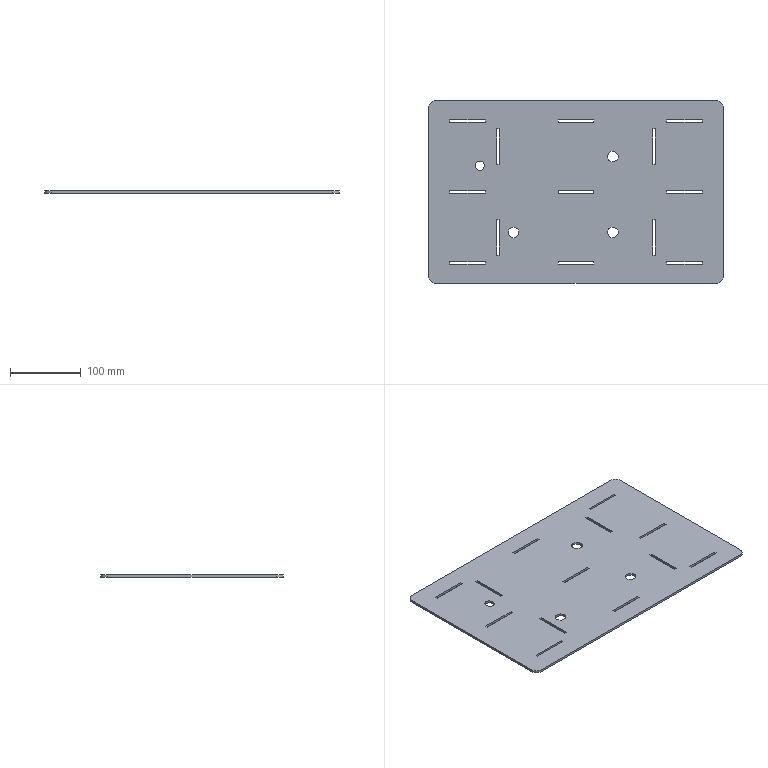Part | SolidWorks | features FlatPattern 1, SMBaseFlange 1, SheetMetal 1 | 1 solid | 70 faces | box 416 x 258 x 3.2 mm | volume 334398 mm3 | plane 58 | cylinder 12 | commonest cylinder face diameters 15 x6 20 x4 13 x2